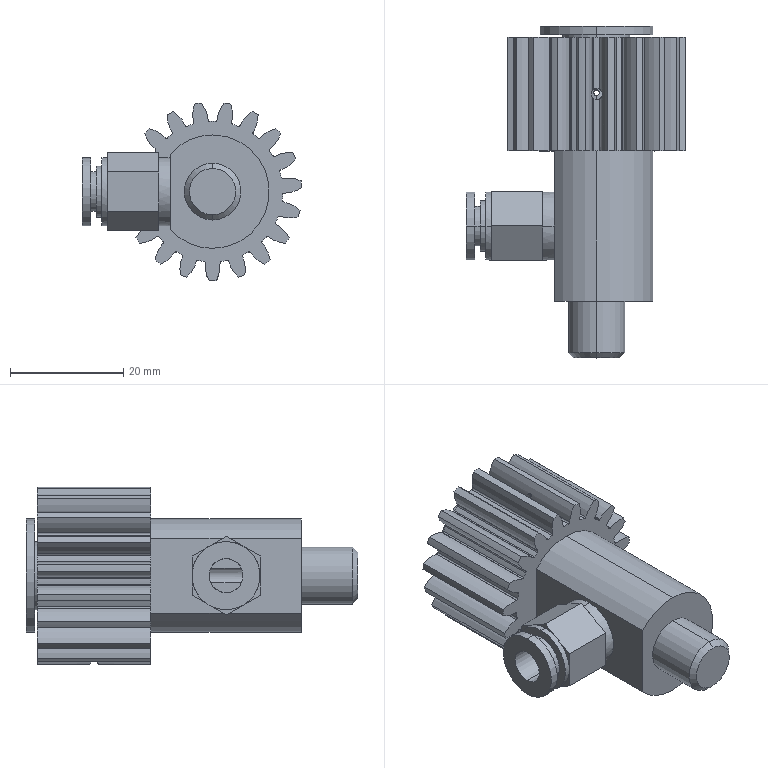Part | SolidWorks | 2 solids | 216 faces | box 38.735 x 58.5 x 31.374 mm | volume 22045 mm3 | cylinder 176 | plane 34 | cone 6 | commonest cylinder face diameters 0.6 x52 12.036 x40 31.5 x22 24.75 x20 12 x12 1 x8